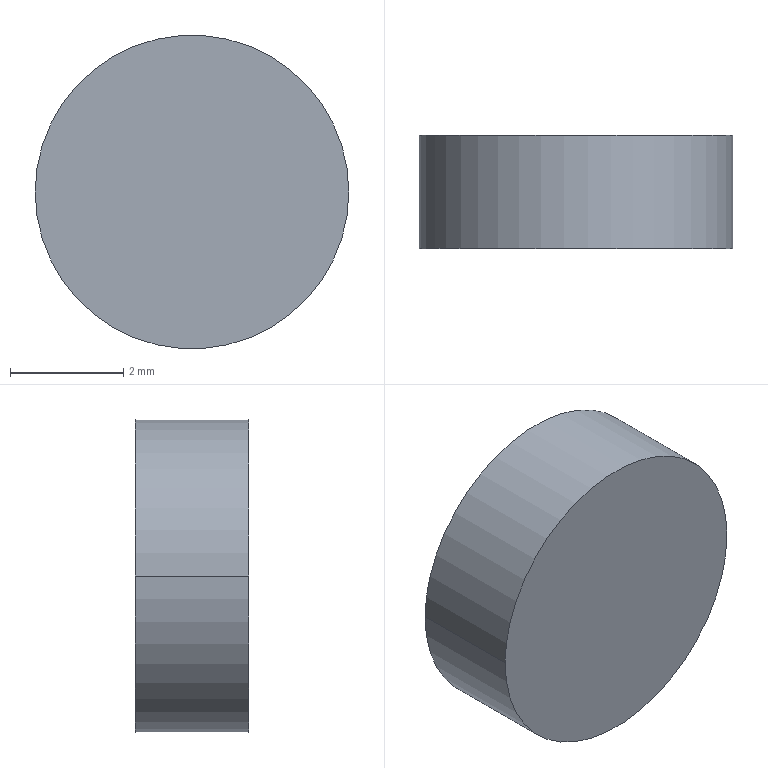Part | SolidWorks | features BaseBody 1 | 1 solid | 11 faces | box 5.54 x 2 x 5.54 mm | volume 44.4 mm3 | plane 9 | cylinder 2 | commonest cylinder face diameters 5.54 x2
STEP:
#1=CARTESIAN_POINT('',(18.23,48.2,-12.25));
#2=VERTEX_POINT('',#1);
#3=CARTESIAN_POINT('',(23.77,48.2,-12.25));
#4=VERTEX_POINT('',#3);
#5=CARTESIAN_POINT('',(21.,48.2,-12.25));
#6=DIRECTION('',(0.,1.,0.));
#7=DIRECTION('',(-1.,0.,0.));
#8=AXIS2_PLACEMENT_3D('',#5,#6,#7);
#9=CIRCLE('',#8,2.77);
#10=EDGE_CURVE('',#2,#4,#9,.T.);
#11=ORIENTED_EDGE('',*,*,#10,.T.);
#12=CARTESIAN_POINT('',(23.77,50.2,-12.25));
#13=VERTEX_POINT('',#12);
#14=CARTESIAN_POINT('',(23.77,48.2,-12.25));
#15=DIRECTION('',(0.,1.,0.));
#16=VECTOR('',#15,1000.);
#17=LINE('',#14,#16);
#18=EDGE_CURVE('',#4,#13,#17,.T.);
#19=ORIENTED_EDGE('',*,*,#18,.T.);
#20=CARTESIAN_POINT('',(18.23,50.2,-12.25));
#21=VERTEX_POINT('',#20);
#22=CARTESIAN_POINT('',(21.,50.2,-12.25));
#23=DIRECTION('',(0.,-1.,0.));
#24=DIRECTION('',(-1.,0.,0.));
#25=AXIS2_PLACEMENT_3D('',#22,#23,#24);
#26=CIRCLE('',#25,2.77);
#27=EDGE_CURVE('',#13,#21,#26,.T.);
#28=ORIENTED_EDGE('',*,*,#27,.T.);
#29=CARTESIAN_POINT('',(18.23,48.2,-12.25));
#30=DIRECTION('',(0.,1.,0.));
#31=VECTOR('',#30,1000.);
#32=LINE('',#29,#31);
#33=EDGE_CURVE('',#2,#21,#32,.T.);
#34=ORIENTED_EDGE('',*,*,#33,.F.);
#35=EDGE_LOOP('',(#11,#19,#28,#34));
#36=FACE_OUTER_BOUND('',#35,.T.);
#37=CARTESIAN_POINT('',(21.,48.2,-12.25));
#38=DIRECTION('',(0.,1.,0.));
#39=DIRECTION('',(-1.,0.,0.));
#40=AXIS2_PLACEMENT_3D('',#37,#38,#39);
#41=CYLINDRICAL_SURFACE('',#40,2.77);
#42=ADVANCED_FACE('',(#36),#41,.T.);
#43=ORIENTED_EDGE('',*,*,#18,.F.);
#44=CARTESIAN_POINT('',(21.,48.2,-12.25));
#45=DIRECTION('',(0.,1.,0.));
#46=DIRECTION('',(-1.,0.,0.));
#47=AXIS2_PLACEMENT_3D('',#44,#45,#46);
#48=CIRCLE('',#47,2.77);
#49=EDGE_CURVE('',#4,#2,#48,.T.);
#50=ORIENTED_EDGE('',*,*,#49,.T.);
#51=ORIENTED_EDGE('',*,*,#33,.T.);
#52=CARTESIAN_POINT('',(21.,50.2,-12.25));
#53=DIRECTION('',(0.,-1.,0.));
#54=DIRECTION('',(-1.,0.,0.));
#55=AXIS2_PLACEMENT_3D('',#52,#53,#54);
#56=CIRCLE('',#55,2.77);
#57=EDGE_CURVE('',#21,#13,#56,.T.);
#58=ORIENTED_EDGE('',*,*,#57,.T.);
#59=EDGE_LOOP('',(#43,#50,#51,#58));
#60=FACE_OUTER_BOUND('',#59,.T.);
#61=CARTESIAN_POINT('',(21.,48.2,-12.25));
#62=DIRECTION('',(0.,1.,0.));
#63=DIRECTION('',(-1.,0.,0.));
#64=AXIS2_PLACEMENT_3D('',#61,#62,#63);
#65=CYLINDRICAL_SURFACE('',#64,2.77);
#66=ADVANCED_FACE('',(#60),#65,.T.);
#67=ORIENTED_EDGE('',*,*,#57,.F.);
#68=ORIENTED_EDGE('',*,*,#27,.F.);
#69=EDGE_LOOP('',(#67,#68));
#70=FACE_OUTER_BOUND('',#69,.T.);
#71=CARTESIAN_POINT('',(22.,50.2,-12.827));
#72=VERTEX_POINT('',#71);
#73=CARTESIAN_POINT('',(22.,50.2,-11.673));
#74=VERTEX_POINT('',#73);
#75=CARTESIAN_POINT('',(22.,50.2,-12.25));
#76=DIRECTION('',(0.,0.,1.));
#77=VECTOR('',#76,1000.);
#78=LINE('',#75,#77);
#79=EDGE_CURVE('',#72,#74,#78,.T.);
#80=ORIENTED_EDGE('',*,*,#79,.T.);
#81=CARTESIAN_POINT('',(21.,50.2,-11.095));
#82=VERTEX_POINT('',#81);
#83=CARTESIAN_POINT('',(22.,50.2,-11.673));
#84=DIRECTION('',(-0.866,0.,0.5));
#85=VECTOR('',#84,1000.);
#86=LINE('',#83,#85);
#87=EDGE_CURVE('',#74,#82,#86,.T.);
#88=ORIENTED_EDGE('',*,*,#87,.T.);
#89=CARTESIAN_POINT('',(20.,50.2,-11.673));
#90=VERTEX_POINT('',#89);
#91=CARTESIAN_POINT('',(21.,50.2,-11.095));
#92=DIRECTION('',(-0.866,0.,-0.5));
#93=VECTOR('',#92,1000.);
#94=LINE('',#91,#93);
#95=EDGE_CURVE('',#82,#90,#94,.T.);
#96=ORIENTED_EDGE('',*,*,#95,.T.);
#97=CARTESIAN_POINT('',(20.,50.2,-12.827));
#98=VERTEX_POINT('',#97);
#99=CARTESIAN_POINT('',(20.,50.2,-12.25));
#100=DIRECTION('',(0.,0.,-1.));
#101=VECTOR('',#100,1000.);
#102=LINE('',#99,#101);
#103=EDGE_CURVE('',#90,#98,#102,.T.);
#104=ORIENTED_EDGE('',*,*,#103,.T.);
#105=CARTESIAN_POINT('',(21.,50.2,-13.405));
#106=VERTEX_POINT('',#105);
#107=CARTESIAN_POINT('',(20.,50.2,-12.827));
#108=DIRECTION('',(0.866,0.,-0.5));
#109=VECTOR('',#108,1000.);
#110=LINE('',#107,#109);
#111=EDGE_CURVE('',#98,#106,#110,.T.);
#112=ORIENTED_EDGE('',*,*,#111,.T.);
#113=CARTESIAN_POINT('',(21.,50.2,-13.405));
#114=DIRECTION('',(0.866,0.,0.5));
#115=VECTOR('',#114,1000.);
#116=LINE('',#113,#115);
#117=EDGE_CURVE('',#106,#72,#116,.T.);
#118=ORIENTED_EDGE('',*,*,#117,.T.);
#119=EDGE_LOOP('',(#80,#88,#96,#104,#112,#118));
#120=FACE_BOUND('',#119,.T.);
#121=CARTESIAN_POINT('',(21.,50.2,-12.25));
#122=DIRECTION('',(0.,1.,0.));
#123=DIRECTION('',(-1.,0.,0.));
#124=AXIS2_PLACEMENT_3D('',#121,#122,#123);
#125=PLANE('',#124);
#126=ADVANCED_FACE('',(#70,#120),#125,.T.);
#127=ORIENTED_EDGE('',*,*,#10,.F.);
#128=ORIENTED_EDGE('',*,*,#49,.F.);
#129=EDGE_LOOP('',(#127,#128));
#130=FACE_OUTER_BOUND('',#129,.T.);
#131=CARTESIAN_POINT('',(21.,48.2,-12.25));
#132=DIRECTION('',(0.,1.,0.));
#133=DIRECTION('',(-1.,0.,0.));
#134=AXIS2_PLACEMENT_3D('',#131,#132,#133);
#135=PLANE('',#134);
#136=ADVANCED_FACE('',(#130),#135,.F.);
#137=CARTESIAN_POINT('',(22.,49.1,-11.673));
#138=VERTEX_POINT('',#137);
#139=CARTESIAN_POINT('',(22.,49.1,-11.673));
#140=DIRECTION('',(0.,1.,0.));
#141=VECTOR('',#140,1000.);
#142=LINE('',#139,#141);
#143=EDGE_CURVE('',#138,#74,#142,.T.);
#144=ORIENTED_EDGE('',*,*,#143,.F.);
#145=CARTESIAN_POINT('',(21.,49.1,-11.095));
#146=VERTEX_POINT('',#145);
#147=CARTESIAN_POINT('',(21.,49.1,-11.095));
#148=DIRECTION('',(0.866,0.,-0.5));
#149=VECTOR('',#148,1000.);
#150=LINE('',#147,#149);
#151=EDGE_CURVE('',#146,#138,#150,.T.);
#152=ORIENTED_EDGE('',*,*,#151,.F.);
#153=CARTESIAN_POINT('',(21.,49.1,-11.095));
#154=DIRECTION('',(0.,-1.,0.));
#155=VECTOR('',#154,1000.);
#156=LINE('',#153,#155);
#157=EDGE_CURVE('',#82,#146,#156,.T.);
#158=ORIENTED_EDGE('',*,*,#157,.F.);
#159=ORIENTED_EDGE('',*,*,#87,.F.);
#160=EDGE_LOOP('',(#144,#152,#158,#159));
#161=FACE_OUTER_BOUND('',#160,.T.);
#162=CARTESIAN_POINT('',(21.,49.1,-11.095));
#163=DIRECTION('',(0.5,0.,0.866));
#164=DIRECTION('',(0.866,0.,-0.5));
#165=AXIS2_PLACEMENT_3D('',#162,#163,#164);
#166=PLANE('',#165);
#167=ADVANCED_FACE('',(#161),#166,.F.);
#168=CARTESIAN_POINT('',(22.,49.1,-12.827));
#169=VERTEX_POINT('',#168);
#170=CARTESIAN_POINT('',(22.,49.1,-12.827));
#171=DIRECTION('',(0.,1.,0.));
#172=VECTOR('',#171,1000.);
#173=LINE('',#170,#172);
#174=EDGE_CURVE('',#169,#72,#173,.T.);
#175=ORIENTED_EDGE('',*,*,#174,.F.);
#176=CARTESIAN_POINT('',(22.,49.1,-11.673));
#177=DIRECTION('',(0.,0.,-1.));
#178=VECTOR('',#177,1000.);
#179=LINE('',#176,#178);
#180=EDGE_CURVE('',#138,#169,#179,.T.);
#181=ORIENTED_EDGE('',*,*,#180,.F.);
#182=ORIENTED_EDGE('',*,*,#143,.T.);
#183=ORIENTED_EDGE('',*,*,#79,.F.);
#184=EDGE_LOOP('',(#175,#181,#182,#183));
#185=FACE_OUTER_BOUND('',#184,.T.);
#186=CARTESIAN_POINT('',(22.,49.1,-11.673));
#187=DIRECTION('',(1.,0.,0.));
#188=DIRECTION('',(0.,1.,0.));
#189=AXIS2_PLACEMENT_3D('',#186,#187,#188);
#190=PLANE('',#189);
#191=ADVANCED_FACE('',(#185),#190,.F.);
#192=CARTESIAN_POINT('',(21.,49.1,-13.405));
#193=VERTEX_POINT('',#192);
#194=CARTESIAN_POINT('',(21.,49.1,-13.405));
#195=DIRECTION('',(0.,1.,0.));
#196=VECTOR('',#195,1000.);
#197=LINE('',#194,#196);
#198=EDGE_CURVE('',#193,#106,#197,.T.);
#199=ORIENTED_EDGE('',*,*,#198,.F.);
#200=CARTESIAN_POINT('',(22.,49.1,-12.827));
#201=DIRECTION('',(-0.866,0.,-0.5));
#202=VECTOR('',#201,1000.);
#203=LINE('',#200,#202);
#204=EDGE_CURVE('',#169,#193,#203,.T.);
#205=ORIENTED_EDGE('',*,*,#204,.F.);
#206=ORIENTED_EDGE('',*,*,#174,.T.);
#207=ORIENTED_EDGE('',*,*,#117,.F.);
#208=EDGE_LOOP('',(#199,#205,#206,#207));
#209=FACE_OUTER_BOUND('',#208,.T.);
#210=CARTESIAN_POINT('',(22.,49.1,-12.827));
#211=DIRECTION('',(0.5,0.,-0.866));
#212=DIRECTION('',(-0.866,0.,-0.5));
#213=AXIS2_PLACEMENT_3D('',#210,#211,#212);
#214=PLANE('',#213);
#215=ADVANCED_FACE('',(#209),#214,.F.);
#216=CARTESIAN_POINT('',(20.,49.1,-12.827));
#217=VERTEX_POINT('',#216);
#218=CARTESIAN_POINT('',(20.,49.1,-12.827));
#219=DIRECTION('',(0.,1.,0.));
#220=VECTOR('',#219,1000.);
#221=LINE('',#218,#220);
#222=EDGE_CURVE('',#217,#98,#221,.T.);
#223=ORIENTED_EDGE('',*,*,#222,.F.);
#224=CARTESIAN_POINT('',(21.,49.1,-13.405));
#225=DIRECTION('',(-0.866,0.,0.5));
#226=VECTOR('',#225,1000.);
#227=LINE('',#224,#226);
#228=EDGE_CURVE('',#193,#217,#227,.T.);
#229=ORIENTED_EDGE('',*,*,#228,.F.);
#230=ORIENTED_EDGE('',*,*,#198,.T.);
#231=ORIENTED_EDGE('',*,*,#111,.F.);
#232=EDGE_LOOP('',(#223,#229,#230,#231));
#233=FACE_OUTER_BOUND('',#232,.T.);
#234=CARTESIAN_POINT('',(21.,49.1,-13.405));
#235=DIRECTION('',(-0.5,0.,-0.866));
#236=DIRECTION('',(-0.866,0.,0.5));
#237=AXIS2_PLACEMENT_3D('',#234,#235,#236);
#238=PLANE('',#237);
#239=ADVANCED_FACE('',(#233),#238,.F.);
#240=CARTESIAN_POINT('',(20.,49.1,-11.673));
#241=VERTEX_POINT('',#240);
#242=CARTESIAN_POINT('',(20.,49.1,-11.673));
#243=DIRECTION('',(0.,1.,0.));
#244=VECTOR('',#243,1000.);
#245=LINE('',#242,#244);
#246=EDGE_CURVE('',#241,#90,#245,.T.);
#247=ORIENTED_EDGE('',*,*,#246,.F.);
#248=CARTESIAN_POINT('',(20.,49.1,-12.827));
#249=DIRECTION('',(0.,0.,1.));
#250=VECTOR('',#249,1000.);
#251=LINE('',#248,#250);
#252=EDGE_CURVE('',#217,#241,#251,.T.);
#253=ORIENTED_EDGE('',*,*,#252,.F.);
#254=ORIENTED_EDGE('',*,*,#222,.T.);
#255=ORIENTED_EDGE('',*,*,#103,.F.);
#256=EDGE_LOOP('',(#247,#253,#254,#255));
#257=FACE_OUTER_BOUND('',#256,.T.);
#258=CARTESIAN_POINT('',(20.,49.1,-12.827));
#259=DIRECTION('',(-1.,0.,0.));
#260=DIRECTION('',(0.,-1.,0.));
#261=AXIS2_PLACEMENT_3D('',#258,#259,#260);
#262=PLANE('',#261);
#263=ADVANCED_FACE('',(#257),#262,.F.);
#264=ORIENTED_EDGE('',*,*,#157,.T.);
#265=CARTESIAN_POINT('',(20.,49.1,-11.673));
#266=DIRECTION('',(0.866,0.,0.5));
#267=VECTOR('',#266,1000.);
#268=LINE('',#265,#267);
#269=EDGE_CURVE('',#241,#146,#268,.T.);
#270=ORIENTED_EDGE('',*,*,#269,.F.);
#271=ORIENTED_EDGE('',*,*,#246,.T.);
#272=ORIENTED_EDGE('',*,*,#95,.F.);
#273=EDGE_LOOP('',(#264,#270,#271,#272));
#274=FACE_OUTER_BOUND('',#273,.T.);
#275=CARTESIAN_POINT('',(20.,49.1,-11.673));
#276=DIRECTION('',(-0.5,0.,0.866));
#277=DIRECTION('',(0.866,0.,0.5));
#278=AXIS2_PLACEMENT_3D('',#275,#276,#277);
#279=PLANE('',#278);
#280=ADVANCED_FACE('',(#274),#279,.F.);
#281=ORIENTED_EDGE('',*,*,#228,.T.);
#282=ORIENTED_EDGE('',*,*,#252,.T.);
#283=ORIENTED_EDGE('',*,*,#269,.T.);
#284=ORIENTED_EDGE('',*,*,#151,.T.);
#285=ORIENTED_EDGE('',*,*,#180,.T.);
#286=ORIENTED_EDGE('',*,*,#204,.T.);
#287=EDGE_LOOP('',(#281,#282,#283,#284,#285,#286));
#288=FACE_OUTER_BOUND('',#287,.T.);
#289=CARTESIAN_POINT('',(0.,49.1,0.));
#290=DIRECTION('',(0.,1.,0.));
#291=DIRECTION('',(0.,0.,1.));
#292=AXIS2_PLACEMENT_3D('',#289,#290,#291);
#293=PLANE('',#292);
#294=ADVANCED_FACE('',(#288),#293,.T.);
#295=CLOSED_SHELL('',(#42,#66,#126,#136,#167,#191,#215,#239,#263,#280,#294));
#296=MANIFOLD_SOLID_BREP('',#295);
#297=CARTESIAN_POINT('',(0.,0.,0.));
#298=DIRECTION('',(0.,0.,1.));
#299=DIRECTION('',(1.,0.,0.));
#300=AXIS2_PLACEMENT_3D('',#297,#298,#299);
#301=(LENGTH_UNIT()NAMED_UNIT(*)SI_UNIT(.MILLI.,.METRE.));
#302=UNCERTAINTY_MEASURE_WITH_UNIT(LENGTH_MEASURE(0.00001),#301,'','');
#303=(NAMED_UNIT(*)PLANE_ANGLE_UNIT()SI_UNIT($,.RADIAN.));
#304=(NAMED_UNIT(*)SI_UNIT($,.STERADIAN.)SOLID_ANGLE_UNIT());
#305=(GEOMETRIC_REPRESENTATION_CONTEXT(3)GLOBAL_UNCERTAINTY_ASSIGNED_CONTEXT((#302))GLOBAL_UNIT_ASSIGNED_CONTEXT((#301,#303,#304))REPRESENTATION_CONTEXT('',''));
#306=ADVANCED_BREP_SHAPE_REPRESENTATION('',(#296,#300),#305);